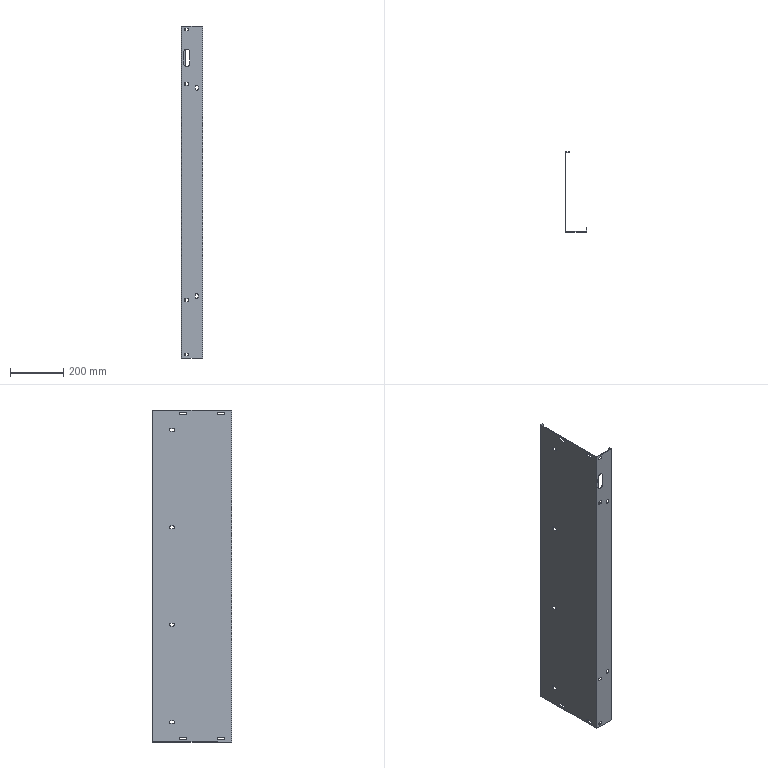Part | SolidWorks | features ICE 11, Cut 6, EdgeFlange 5, SMBaseFlange 4, Chamfer 1, FlatPattern 1, LPattern 1, SheetMetal 1 | 1 solid | 121 faces | box 80 x 299.5 x 1250 mm | volume 750751 mm3 | plane 74 | cylinder 47 | commonest cylinder face diameters 10 x16 9 x12 11 x10 0.4 x3 3.4 x3 24 x3